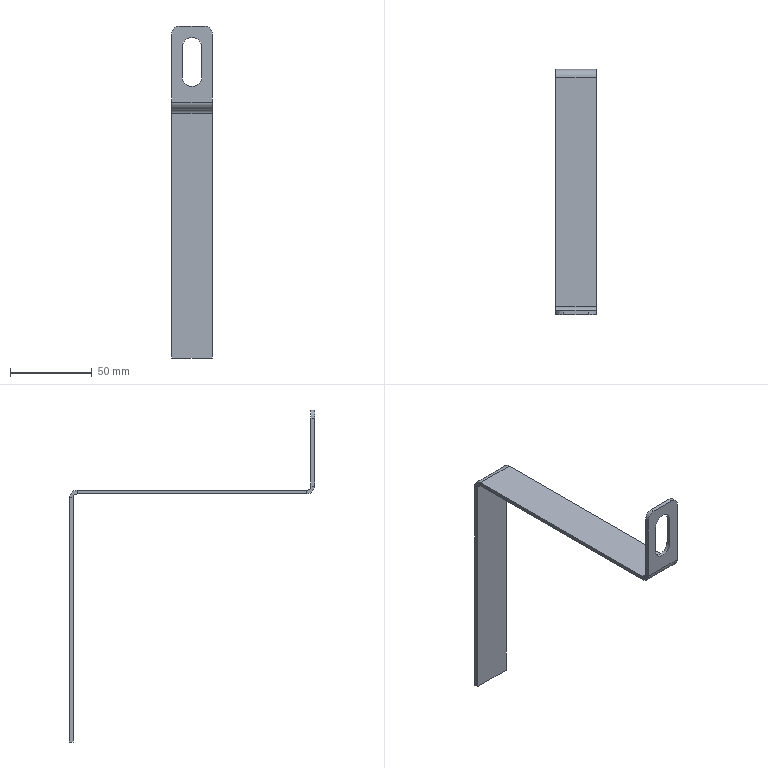Part | SolidWorks | features Fillet 1, FlatPattern 1, ICE 1, SMBaseFlange 1, SheetMetal 1 | 1 solid | 29 faces | box 25 x 150 x 203 mm | volume 19203 mm3 | plane 20 | cylinder 9 | commonest cylinder face diameters 12 x3 5 x2 9.6 x2 10 x2
STEP:
#1=CARTESIAN_POINT('',(6.,-2.3,-13.));
#2=VERTEX_POINT('',#1);
#3=CARTESIAN_POINT('',(0.,-2.3,-7.));
#4=VERTEX_POINT('',#3);
#5=CARTESIAN_POINT('',(0.,-2.3,-13.));
#6=DIRECTION('',(0.,-1.,0.));
#7=DIRECTION('',(0.,0.,1.));
#8=AXIS2_PLACEMENT_3D('',#5,#6,#7);
#9=CIRCLE('',#8,6.);
#10=EDGE_CURVE('',#2,#4,#9,.T.);
#11=ORIENTED_EDGE('',*,*,#10,.T.);
#12=CARTESIAN_POINT('',(0.,0.,-7.));
#13=VERTEX_POINT('',#12);
#14=CARTESIAN_POINT('',(0.,-2.301,-7.));
#15=DIRECTION('',(0.,1.,0.));
#16=VECTOR('',#15,1000.);
#17=LINE('',#14,#16);
#18=EDGE_CURVE('',#4,#13,#17,.T.);
#19=ORIENTED_EDGE('',*,*,#18,.T.);
#20=CARTESIAN_POINT('',(6.,0.,-13.));
#21=VERTEX_POINT('',#20);
#22=CARTESIAN_POINT('',(0.,0.,-13.));
#23=DIRECTION('',(0.,1.,0.));
#24=DIRECTION('',(0.,0.,1.));
#25=AXIS2_PLACEMENT_3D('',#22,#23,#24);
#26=CIRCLE('',#25,6.);
#27=EDGE_CURVE('',#13,#21,#26,.T.);
#28=ORIENTED_EDGE('',*,*,#27,.T.);
#29=CARTESIAN_POINT('',(6.,-2.301,-13.));
#30=DIRECTION('',(0.,1.,0.));
#31=VECTOR('',#30,1000.);
#32=LINE('',#29,#31);
#33=EDGE_CURVE('',#2,#21,#32,.T.);
#34=ORIENTED_EDGE('',*,*,#33,.F.);
#35=EDGE_LOOP('',(#11,#19,#28,#34));
#36=FACE_OUTER_BOUND('',#35,.T.);
#37=CARTESIAN_POINT('',(0.,-2.301,-13.));
#38=DIRECTION('',(0.,1.,0.));
#39=DIRECTION('',(0.,0.,1.));
#40=AXIS2_PLACEMENT_3D('',#37,#38,#39);
#41=CYLINDRICAL_SURFACE('',#40,6.);
#42=ADVANCED_FACE('',(#36),#41,.F.);
#43=CARTESIAN_POINT('',(12.5,2.5,-49.));
#44=VERTEX_POINT('',#43);
#45=CARTESIAN_POINT('',(12.5,2.5,-51.3));
#46=VERTEX_POINT('',#45);
#47=CARTESIAN_POINT('',(12.5,2.5,-49.));
#48=DIRECTION('',(0.,0.,-1.));
#49=VECTOR('',#48,1000.);
#50=LINE('',#47,#49);
#51=EDGE_CURVE('',#44,#46,#50,.T.);
#52=ORIENTED_EDGE('',*,*,#51,.F.);
#53=CARTESIAN_POINT('',(12.5,0.,-46.5));
#54=VERTEX_POINT('',#53);
#55=CARTESIAN_POINT('',(12.5,2.5,-46.5));
#56=DIRECTION('',(1.,0.,0.));
#57=DIRECTION('',(0.,0.,1.));
#58=AXIS2_PLACEMENT_3D('',#55,#56,#57);
#59=CIRCLE('',#58,2.5);
#60=EDGE_CURVE('',#54,#44,#59,.T.);
#61=ORIENTED_EDGE('',*,*,#60,.F.);
#62=CARTESIAN_POINT('',(12.5,-2.3,-46.5));
#63=VERTEX_POINT('',#62);
#64=CARTESIAN_POINT('',(12.5,-2.3,-46.5));
#65=DIRECTION('',(0.,1.,0.));
#66=VECTOR('',#65,1000.);
#67=LINE('',#64,#66);
#68=EDGE_CURVE('',#63,#54,#67,.T.);
#69=ORIENTED_EDGE('',*,*,#68,.F.);
#70=CARTESIAN_POINT('',(12.5,2.5,-46.5));
#71=DIRECTION('',(1.,0.,0.));
#72=DIRECTION('',(0.,0.,-1.));
#73=AXIS2_PLACEMENT_3D('',#70,#71,#72);
#74=CIRCLE('',#73,4.8);
#75=EDGE_CURVE('',#63,#46,#74,.T.);
#76=ORIENTED_EDGE('',*,*,#75,.T.);
#77=EDGE_LOOP('',(#52,#61,#69,#76));
#78=FACE_OUTER_BOUND('',#77,.T.);
#79=CARTESIAN_POINT('',(12.5,2.5,-49.));
#80=DIRECTION('',(1.,0.,0.));
#81=DIRECTION('',(0.,0.,-1.));
#82=AXIS2_PLACEMENT_3D('',#79,#80,#81);
#83=PLANE('',#82);
#84=ADVANCED_FACE('',(#78),#83,.T.);
#85=CARTESIAN_POINT('',(12.5,142.9,-49.));
#86=VERTEX_POINT('',#85);
#87=CARTESIAN_POINT('',(12.5,0.,-49.));
#88=DIRECTION('',(0.,1.,0.));
#89=VECTOR('',#88,1000.);
#90=LINE('',#87,#89);
#91=EDGE_CURVE('',#44,#86,#90,.T.);
#92=ORIENTED_EDGE('',*,*,#91,.F.);
#93=ORIENTED_EDGE('',*,*,#51,.T.);
#94=CARTESIAN_POINT('',(12.5,142.9,-51.3));
#95=VERTEX_POINT('',#94);
#96=CARTESIAN_POINT('',(12.5,0.,-51.3));
#97=DIRECTION('',(0.,1.,0.));
#98=VECTOR('',#97,1000.);
#99=LINE('',#96,#98);
#100=EDGE_CURVE('',#46,#95,#99,.T.);
#101=ORIENTED_EDGE('',*,*,#100,.T.);
#102=CARTESIAN_POINT('',(12.5,142.9,-51.3));
#103=DIRECTION('',(0.,0.,1.));
#104=VECTOR('',#103,1000.);
#105=LINE('',#102,#104);
#106=EDGE_CURVE('',#95,#86,#105,.T.);
#107=ORIENTED_EDGE('',*,*,#106,.T.);
#108=EDGE_LOOP('',(#92,#93,#101,#107));
#109=FACE_OUTER_BOUND('',#108,.T.);
#110=CARTESIAN_POINT('',(12.5,-2.3,-46.5));
#111=DIRECTION('',(1.,0.,0.));
#112=DIRECTION('',(0.,0.,-1.));
#113=AXIS2_PLACEMENT_3D('',#110,#111,#112);
#114=PLANE('',#113);
#115=ADVANCED_FACE('',(#109),#114,.T.);
#116=CARTESIAN_POINT('',(-12.5,0.,-46.5));
#117=VERTEX_POINT('',#116);
#118=CARTESIAN_POINT('',(-12.5,-2.3,-46.5));
#119=VERTEX_POINT('',#118);
#120=CARTESIAN_POINT('',(-12.5,0.,-46.5));
#121=DIRECTION('',(0.,-1.,0.));
#122=VECTOR('',#121,1000.);
#123=LINE('',#120,#122);
#124=EDGE_CURVE('',#117,#119,#123,.T.);
#125=ORIENTED_EDGE('',*,*,#124,.F.);
#126=CARTESIAN_POINT('',(-12.5,2.5,-49.));
#127=VERTEX_POINT('',#126);
#128=CARTESIAN_POINT('',(-12.5,2.5,-46.5));
#129=DIRECTION('',(1.,0.,0.));
#130=DIRECTION('',(0.,0.,1.));
#131=AXIS2_PLACEMENT_3D('',#128,#129,#130);
#132=CIRCLE('',#131,2.5);
#133=EDGE_CURVE('',#117,#127,#132,.T.);
#134=ORIENTED_EDGE('',*,*,#133,.T.);
#135=CARTESIAN_POINT('',(-12.5,2.5,-51.3));
#136=VERTEX_POINT('',#135);
#137=CARTESIAN_POINT('',(-12.5,2.5,-51.3));
#138=DIRECTION('',(0.,0.,1.));
#139=VECTOR('',#138,1000.);
#140=LINE('',#137,#139);
#141=EDGE_CURVE('',#136,#127,#140,.T.);
#142=ORIENTED_EDGE('',*,*,#141,.F.);
#143=CARTESIAN_POINT('',(-12.5,2.5,-46.5));
#144=DIRECTION('',(1.,0.,0.));
#145=DIRECTION('',(0.,0.,-1.));
#146=AXIS2_PLACEMENT_3D('',#143,#144,#145);
#147=CIRCLE('',#146,4.8);
#148=EDGE_CURVE('',#119,#136,#147,.T.);
#149=ORIENTED_EDGE('',*,*,#148,.F.);
#150=EDGE_LOOP('',(#125,#134,#142,#149));
#151=FACE_OUTER_BOUND('',#150,.T.);
#152=CARTESIAN_POINT('',(-12.5,0.,-46.5));
#153=DIRECTION('',(-1.,0.,0.));
#154=DIRECTION('',(0.,0.,1.));
#155=AXIS2_PLACEMENT_3D('',#152,#153,#154);
#156=PLANE('',#155);
#157=ADVANCED_FACE('',(#151),#156,.T.);
#158=CARTESIAN_POINT('',(-12.5,-2.3,-5.));
#159=VERTEX_POINT('',#158);
#160=CARTESIAN_POINT('',(-12.5,-2.3,0.));
#161=DIRECTION('',(0.,0.,-1.));
#162=VECTOR('',#161,1000.);
#163=LINE('',#160,#162);
#164=EDGE_CURVE('',#159,#119,#163,.T.);
#165=ORIENTED_EDGE('',*,*,#164,.F.);
#166=CARTESIAN_POINT('',(-12.5,0.,-5.));
#167=VERTEX_POINT('',#166);
#168=CARTESIAN_POINT('',(-12.5,2.5,-5.));
#169=DIRECTION('',(0.,1.,0.));
#170=VECTOR('',#169,1000.);
#171=LINE('',#168,#170);
#172=EDGE_CURVE('',#159,#167,#171,.T.);
#173=ORIENTED_EDGE('',*,*,#172,.T.);
#174=CARTESIAN_POINT('',(-12.5,0.,0.));
#175=DIRECTION('',(0.,0.,-1.));
#176=VECTOR('',#175,1000.);
#177=LINE('',#174,#176);
#178=EDGE_CURVE('',#167,#117,#177,.T.);
#179=ORIENTED_EDGE('',*,*,#178,.T.);
#180=ORIENTED_EDGE('',*,*,#124,.T.);
#181=EDGE_LOOP('',(#165,#173,#179,#180));
#182=FACE_OUTER_BOUND('',#181,.T.);
#183=CARTESIAN_POINT('',(-12.5,2.5,-51.3));
#184=DIRECTION('',(-1.,0.,0.));
#185=DIRECTION('',(0.,0.,1.));
#186=AXIS2_PLACEMENT_3D('',#183,#184,#185);
#187=PLANE('',#186);
#188=ADVANCED_FACE('',(#182),#187,.T.);
#189=CARTESIAN_POINT('',(12.5,147.7,-53.8));
#190=VERTEX_POINT('',#189);
#191=CARTESIAN_POINT('',(12.5,145.4,-53.8));
#192=VERTEX_POINT('',#191);
#193=CARTESIAN_POINT('',(12.5,147.7,-53.8));
#194=DIRECTION('',(0.,-1.,0.));
#195=VECTOR('',#194,1000.);
#196=LINE('',#193,#195);
#197=EDGE_CURVE('',#190,#192,#196,.T.);
#198=ORIENTED_EDGE('',*,*,#197,.F.);
#199=CARTESIAN_POINT('',(12.5,142.9,-53.8));
#200=DIRECTION('',(-1.,0.,0.));
#201=DIRECTION('',(0.,0.,-1.));
#202=AXIS2_PLACEMENT_3D('',#199,#200,#201);
#203=CIRCLE('',#202,4.8);
#204=EDGE_CURVE('',#86,#190,#203,.T.);
#205=ORIENTED_EDGE('',*,*,#204,.F.);
#206=ORIENTED_EDGE('',*,*,#106,.F.);
#207=CARTESIAN_POINT('',(12.5,142.9,-53.8));
#208=DIRECTION('',(-1.,0.,0.));
#209=DIRECTION('',(0.,0.,-1.));
#210=AXIS2_PLACEMENT_3D('',#207,#208,#209);
#211=CIRCLE('',#210,2.5);
#212=EDGE_CURVE('',#95,#192,#211,.T.);
#213=ORIENTED_EDGE('',*,*,#212,.T.);
#214=EDGE_LOOP('',(#198,#205,#206,#213));
#215=FACE_OUTER_BOUND('',#214,.T.);
#216=CARTESIAN_POINT('',(12.5,147.7,-53.8));
#217=DIRECTION('',(1.,0.,0.));
#218=DIRECTION('',(0.,0.,-1.));
#219=AXIS2_PLACEMENT_3D('',#216,#217,#218);
#220=PLANE('',#219);
#221=ADVANCED_FACE('',(#215),#220,.T.);
#222=CARTESIAN_POINT('',(12.5,147.7,-203.));
#223=VERTEX_POINT('',#222);
#224=CARTESIAN_POINT('',(12.5,147.7,-49.));
#225=DIRECTION('',(0.,0.,-1.));
#226=VECTOR('',#225,1000.);
#227=LINE('',#224,#226);
#228=EDGE_CURVE('',#190,#223,#227,.T.);
#229=ORIENTED_EDGE('',*,*,#228,.F.);
#230=ORIENTED_EDGE('',*,*,#197,.T.);
#231=CARTESIAN_POINT('',(12.5,145.4,-203.));
#232=VERTEX_POINT('',#231);
#233=CARTESIAN_POINT('',(12.5,145.4,-49.));
#234=DIRECTION('',(0.,0.,-1.));
#235=VECTOR('',#234,1000.);
#236=LINE('',#233,#235);
#237=EDGE_CURVE('',#192,#232,#236,.T.);
#238=ORIENTED_EDGE('',*,*,#237,.T.);
#239=CARTESIAN_POINT('',(12.5,147.7,-203.));
#240=DIRECTION('',(0.,-1.,0.));
#241=VECTOR('',#240,1000.);
#242=LINE('',#239,#241);
#243=EDGE_CURVE('',#223,#232,#242,.T.);
#244=ORIENTED_EDGE('',*,*,#243,.F.);
#245=EDGE_LOOP('',(#229,#230,#238,#244));
#246=FACE_OUTER_BOUND('',#245,.T.);
#247=CARTESIAN_POINT('',(12.5,142.9,-51.3));
#248=DIRECTION('',(1.,0.,0.));
#249=DIRECTION('',(0.,0.,-1.));
#250=AXIS2_PLACEMENT_3D('',#247,#248,#249);
#251=PLANE('',#250);
#252=ADVANCED_FACE('',(#246),#251,.T.);
#253=CARTESIAN_POINT('',(-12.5,142.9,-49.));
#254=VERTEX_POINT('',#253);
#255=CARTESIAN_POINT('',(-12.5,142.9,-51.3));
#256=VERTEX_POINT('',#255);
#257=CARTESIAN_POINT('',(-12.5,142.9,-49.));
#258=DIRECTION('',(0.,0.,-1.));
#259=VECTOR('',#258,1000.);
#260=LINE('',#257,#259);
#261=EDGE_CURVE('',#254,#256,#260,.T.);
#262=ORIENTED_EDGE('',*,*,#261,.F.);
#263=CARTESIAN_POINT('',(-12.5,147.7,-53.8));
#264=VERTEX_POINT('',#263);
#265=CARTESIAN_POINT('',(-12.5,142.9,-53.8));
#266=DIRECTION('',(-1.,0.,0.));
#267=DIRECTION('',(0.,0.,-1.));
#268=AXIS2_PLACEMENT_3D('',#265,#266,#267);
#269=CIRCLE('',#268,4.8);
#270=EDGE_CURVE('',#254,#264,#269,.T.);
#271=ORIENTED_EDGE('',*,*,#270,.T.);
#272=CARTESIAN_POINT('',(-12.5,145.4,-53.8));
#273=VERTEX_POINT('',#272);
#274=CARTESIAN_POINT('',(-12.5,145.4,-53.8));
#275=DIRECTION('',(0.,1.,0.));
#276=VECTOR('',#275,1000.);
#277=LINE('',#274,#276);
#278=EDGE_CURVE('',#273,#264,#277,.T.);
#279=ORIENTED_EDGE('',*,*,#278,.F.);
#280=CARTESIAN_POINT('',(-12.5,142.9,-53.8));
#281=DIRECTION('',(-1.,0.,0.));
#282=DIRECTION('',(0.,0.,-1.));
#283=AXIS2_PLACEMENT_3D('',#280,#281,#282);
#284=CIRCLE('',#283,2.5);
#285=EDGE_CURVE('',#256,#273,#284,.T.);
#286=ORIENTED_EDGE('',*,*,#285,.F.);
#287=EDGE_LOOP('',(#262,#271,#279,#286));
#288=FACE_OUTER_BOUND('',#287,.T.);
#289=CARTESIAN_POINT('',(-12.5,142.9,-49.));
#290=DIRECTION('',(-1.,0.,0.));
#291=DIRECTION('',(0.,0.,1.));
#292=AXIS2_PLACEMENT_3D('',#289,#290,#291);
#293=PLANE('',#292);
#294=ADVANCED_FACE('',(#288),#293,.T.);
#295=CARTESIAN_POINT('',(-12.5,0.,-49.));
#296=DIRECTION('',(0.,1.,0.));
#297=VECTOR('',#296,1000.);
#298=LINE('',#295,#297);
#299=EDGE_CURVE('',#127,#254,#298,.T.);
#300=ORIENTED_EDGE('',*,*,#299,.T.);
#301=ORIENTED_EDGE('',*,*,#261,.T.);
#302=CARTESIAN_POINT('',(-12.5,0.,-51.3));
#303=DIRECTION('',(0.,1.,0.));
#304=VECTOR('',#303,1000.);
#305=LINE('',#302,#304);
#306=EDGE_CURVE('',#136,#256,#305,.T.);
#307=ORIENTED_EDGE('',*,*,#306,.F.);
#308=ORIENTED_EDGE('',*,*,#141,.T.);
#309=EDGE_LOOP('',(#300,#301,#307,#308));
#310=FACE_OUTER_BOUND('',#309,.T.);
#311=CARTESIAN_POINT('',(-12.5,145.4,-53.8));
#312=DIRECTION('',(-1.,0.,0.));
#313=DIRECTION('',(0.,0.,1.));
#314=AXIS2_PLACEMENT_3D('',#311,#312,#313);
#315=PLANE('',#314);
#316=ADVANCED_FACE('',(#310),#315,.T.);
#317=CARTESIAN_POINT('',(-12.5,145.4,-203.));
#318=VERTEX_POINT('',#317);
#319=CARTESIAN_POINT('',(-12.5,145.4,-49.));
#320=DIRECTION('',(0.,0.,-1.));
#321=VECTOR('',#320,1000.);
#322=LINE('',#319,#321);
#323=EDGE_CURVE('',#273,#318,#322,.T.);
#324=ORIENTED_EDGE('',*,*,#323,.T.);
#325=CARTESIAN_POINT('',(12.5,145.4,-203.));
#326=DIRECTION('',(-1.,0.,0.));
#327=VECTOR('',#326,1000.);
#328=LINE('',#325,#327);
#329=EDGE_CURVE('',#232,#318,#328,.T.);
#330=ORIENTED_EDGE('',*,*,#329,.F.);
#331=ORIENTED_EDGE('',*,*,#237,.F.);
#332=CARTESIAN_POINT('',(12.5,145.4,-53.8));
#333=DIRECTION('',(-1.,0.,0.));
#334=VECTOR('',#333,1000.);
#335=LINE('',#332,#334);
#336=EDGE_CURVE('',#192,#273,#335,.T.);
#337=ORIENTED_EDGE('',*,*,#336,.T.);
#338=EDGE_LOOP('',(#324,#330,#331,#337));
#339=FACE_OUTER_BOUND('',#338,.T.);
#340=CARTESIAN_POINT('',(12.5,145.4,-49.));
#341=DIRECTION('',(0.,1.,0.));
#342=DIRECTION('',(0.,0.,1.));
#343=AXIS2_PLACEMENT_3D('',#340,#341,#342);
#344=PLANE('',#343);
#345=ADVANCED_FACE('',(#339),#344,.F.);
#346=CARTESIAN_POINT('',(-12.5,147.7,-203.));
#347=VERTEX_POINT('',#346);
#348=CARTESIAN_POINT('',(-12.5,147.7,-203.));
#349=DIRECTION('',(0.,-1.,0.));
#350=VECTOR('',#349,1000.);
#351=LINE('',#348,#350);
#352=EDGE_CURVE('',#347,#318,#351,.T.);
#353=ORIENTED_EDGE('',*,*,#352,.F.);
#354=CARTESIAN_POINT('',(12.5,147.7,-203.));
#355=DIRECTION('',(-1.,0.,0.));
#356=VECTOR('',#355,1000.);
#357=LINE('',#354,#356);
#358=EDGE_CURVE('',#223,#347,#357,.T.);
#359=ORIENTED_EDGE('',*,*,#358,.F.);
#360=ORIENTED_EDGE('',*,*,#243,.T.);
#361=ORIENTED_EDGE('',*,*,#329,.T.);
#362=EDGE_LOOP('',(#353,#359,#360,#361));
#363=FACE_OUTER_BOUND('',#362,.T.);
#364=CARTESIAN_POINT('',(12.5,147.7,-203.));
#365=DIRECTION('',(0.,0.,-1.));
#366=DIRECTION('',(-1.,0.,0.));
#367=AXIS2_PLACEMENT_3D('',#364,#365,#366);
#368=PLANE('',#367);
#369=ADVANCED_FACE('',(#363),#368,.T.);
#370=CARTESIAN_POINT('',(-12.5,147.7,-49.));
#371=DIRECTION('',(0.,0.,-1.));
#372=VECTOR('',#371,1000.);
#373=LINE('',#370,#372);
#374=EDGE_CURVE('',#264,#347,#373,.T.);
#375=ORIENTED_EDGE('',*,*,#374,.F.);
#376=CARTESIAN_POINT('',(12.5,147.7,-53.8));
#377=DIRECTION('',(-1.,0.,0.));
#378=VECTOR('',#377,1000.);
#379=LINE('',#376,#378);
#380=EDGE_CURVE('',#190,#264,#379,.T.);
#381=ORIENTED_EDGE('',*,*,#380,.F.);
#382=ORIENTED_EDGE('',*,*,#228,.T.);
#383=ORIENTED_EDGE('',*,*,#358,.T.);
#384=EDGE_LOOP('',(#375,#381,#382,#383));
#385=FACE_OUTER_BOUND('',#384,.T.);
#386=CARTESIAN_POINT('',(12.5,147.7,-49.));
#387=DIRECTION('',(0.,1.,0.));
#388=DIRECTION('',(0.,0.,1.));
#389=AXIS2_PLACEMENT_3D('',#386,#387,#388);
#390=PLANE('',#389);
#391=ADVANCED_FACE('',(#385),#390,.T.);
#392=ORIENTED_EDGE('',*,*,#270,.F.);
#393=CARTESIAN_POINT('',(12.5,142.9,-49.));
#394=DIRECTION('',(-1.,0.,0.));
#395=VECTOR('',#394,1000.);
#396=LINE('',#393,#395);
#397=EDGE_CURVE('',#86,#254,#396,.T.);
#398=ORIENTED_EDGE('',*,*,#397,.F.);
#399=ORIENTED_EDGE('',*,*,#204,.T.);
#400=ORIENTED_EDGE('',*,*,#380,.T.);
#401=EDGE_LOOP('',(#392,#398,#399,#400));
#402=FACE_OUTER_BOUND('',#401,.T.);
#403=CARTESIAN_POINT('',(12.5,142.9,-53.8));
#404=DIRECTION('',(-1.,0.,0.));
#405=DIRECTION('',(0.,0.,1.));
#406=AXIS2_PLACEMENT_3D('',#403,#404,#405);
#407=CYLINDRICAL_SURFACE('',#406,4.8);
#408=ADVANCED_FACE('',(#402),#407,.T.);
#409=ORIENTED_EDGE('',*,*,#299,.F.);
#410=CARTESIAN_POINT('',(12.5,2.5,-49.));
#411=DIRECTION('',(-1.,0.,0.));
#412=VECTOR('',#411,1000.);
#413=LINE('',#410,#412);
#414=EDGE_CURVE('',#44,#127,#413,.T.);
#415=ORIENTED_EDGE('',*,*,#414,.F.);
#416=ORIENTED_EDGE('',*,*,#91,.T.);
#417=ORIENTED_EDGE('',*,*,#397,.T.);
#418=EDGE_LOOP('',(#409,#415,#416,#417));
#419=FACE_OUTER_BOUND('',#418,.T.);
#420=CARTESIAN_POINT('',(12.5,0.,-49.));
#421=DIRECTION('',(0.,0.,1.));
#422=DIRECTION('',(1.,0.,0.));
#423=AXIS2_PLACEMENT_3D('',#420,#421,#422);
#424=PLANE('',#423);
#425=ADVANCED_FACE('',(#419),#424,.T.);
#426=ORIENTED_EDGE('',*,*,#133,.F.);
#427=CARTESIAN_POINT('',(12.5,0.,-46.5));
#428=DIRECTION('',(-1.,0.,0.));
#429=VECTOR('',#428,1000.);
#430=LINE('',#427,#429);
#431=EDGE_CURVE('',#54,#117,#430,.T.);
#432=ORIENTED_EDGE('',*,*,#431,.F.);
#433=ORIENTED_EDGE('',*,*,#60,.T.);
#434=ORIENTED_EDGE('',*,*,#414,.T.);
#435=EDGE_LOOP('',(#426,#432,#433,#434));
#436=FACE_OUTER_BOUND('',#435,.T.);
#437=CARTESIAN_POINT('',(12.5,2.5,-46.5));
#438=DIRECTION('',(-1.,0.,0.));
#439=DIRECTION('',(0.,0.,1.));
#440=AXIS2_PLACEMENT_3D('',#437,#438,#439);
#441=CYLINDRICAL_SURFACE('',#440,2.5);
#442=ADVANCED_FACE('',(#436),#441,.F.);
#443=CARTESIAN_POINT('',(6.,0.,-31.));
#444=VERTEX_POINT('',#443);
#445=CARTESIAN_POINT('',(-6.,0.,-31.));
#446=VERTEX_POINT('',#445);
#447=CARTESIAN_POINT('',(0.,0.,-31.));
#448=DIRECTION('',(0.,1.,0.));
#449=DIRECTION('',(0.,0.,1.));
#450=AXIS2_PLACEMENT_3D('',#447,#448,#449);
#451=CIRCLE('',#450,6.);
#452=EDGE_CURVE('',#444,#446,#451,.T.);
#453=ORIENTED_EDGE('',*,*,#452,.F.);
#454=CARTESIAN_POINT('',(6.,0.,-31.));
#455=DIRECTION('',(0.,0.,-1.));
#456=VECTOR('',#455,1000.);
#457=LINE('',#454,#456);
#458=EDGE_CURVE('',#21,#444,#457,.T.);
#459=ORIENTED_EDGE('',*,*,#458,.F.);
#460=ORIENTED_EDGE('',*,*,#27,.F.);
#461=CARTESIAN_POINT('',(-6.,0.,-13.));
#462=VERTEX_POINT('',#461);
#463=CARTESIAN_POINT('',(0.,0.,-13.));
#464=DIRECTION('',(0.,1.,0.));
#465=DIRECTION('',(0.,0.,1.));
#466=AXIS2_PLACEMENT_3D('',#463,#464,#465);
#467=CIRCLE('',#466,6.);
#468=EDGE_CURVE('',#462,#13,#467,.T.);
#469=ORIENTED_EDGE('',*,*,#468,.F.);
#470=CARTESIAN_POINT('',(-6.,0.,-31.));
#471=DIRECTION('',(0.,0.,1.));
#472=VECTOR('',#471,1000.);
#473=LINE('',#470,#472);
#474=EDGE_CURVE('',#446,#462,#473,.T.);
#475=ORIENTED_EDGE('',*,*,#474,.F.);
#476=EDGE_LOOP('',(#453,#459,#460,#469,#475));
#477=FACE_BOUND('',#476,.T.);
#478=CARTESIAN_POINT('',(7.5,0.,0.));
#479=VERTEX_POINT('',#478);
#480=CARTESIAN_POINT('',(-7.5,0.,0.));
#481=VERTEX_POINT('',#480);
#482=CARTESIAN_POINT('',(12.5,0.,0.));
#483=DIRECTION('',(-1.,0.,0.));
#484=VECTOR('',#483,1000.);
#485=LINE('',#482,#484);
#486=EDGE_CURVE('',#479,#481,#485,.T.);
#487=ORIENTED_EDGE('',*,*,#486,.F.);
#488=CARTESIAN_POINT('',(12.5,0.,-5.));
#489=VERTEX_POINT('',#488);
#490=CARTESIAN_POINT('',(7.5,0.,-5.));
#491=DIRECTION('',(0.,1.,0.));
#492=DIRECTION('',(0.,0.,1.));
#493=AXIS2_PLACEMENT_3D('',#490,#491,#492);
#494=CIRCLE('',#493,5.);
#495=EDGE_CURVE('',#479,#489,#494,.T.);
#496=ORIENTED_EDGE('',*,*,#495,.T.);
#497=CARTESIAN_POINT('',(12.5,0.,0.));
#498=DIRECTION('',(0.,0.,-1.));
#499=VECTOR('',#498,1000.);
#500=LINE('',#497,#499);
#501=EDGE_CURVE('',#489,#54,#500,.T.);
#502=ORIENTED_EDGE('',*,*,#501,.T.);
#503=ORIENTED_EDGE('',*,*,#431,.T.);
#504=ORIENTED_EDGE('',*,*,#178,.F.);
#505=CARTESIAN_POINT('',(-7.5,0.,-5.));
#506=DIRECTION('',(0.,1.,0.));
#507=DIRECTION('',(0.,0.,1.));
#508=AXIS2_PLACEMENT_3D('',#505,#506,#507);
#509=CIRCLE('',#508,5.);
#510=EDGE_CURVE('',#167,#481,#509,.T.);
#511=ORIENTED_EDGE('',*,*,#510,.T.);
#512=EDGE_LOOP('',(#487,#496,#502,#503,#504,#511));
#513=FACE_OUTER_BOUND('',#512,.T.);
#514=CARTESIAN_POINT('',(12.5,0.,0.));
#515=DIRECTION('',(0.,1.,0.));
#516=DIRECTION('',(0.,0.,1.));
#517=AXIS2_PLACEMENT_3D('',#514,#515,#516);
#518=PLANE('',#517);
#519=ADVANCED_FACE('',(#477,#513),#518,.T.);
#520=CARTESIAN_POINT('',(7.5,-2.3,0.));
#521=VERTEX_POINT('',#520);
#522=CARTESIAN_POINT('',(-7.5,-2.3,0.));
#523=VERTEX_POINT('',#522);
#524=CARTESIAN_POINT('',(12.5,-2.3,0.));
#525=DIRECTION('',(-1.,0.,0.));
#526=VECTOR('',#525,1000.);
#527=LINE('',#524,#526);
#528=EDGE_CURVE('',#521,#523,#527,.T.);
#529=ORIENTED_EDGE('',*,*,#528,.F.);
#530=CARTESIAN_POINT('',(7.5,-2.3,0.));
#531=DIRECTION('',(0.,1.,0.));
#532=VECTOR('',#531,1000.);
#533=LINE('',#530,#532);
#534=EDGE_CURVE('',#521,#479,#533,.T.);
#535=ORIENTED_EDGE('',*,*,#534,.T.);
#536=ORIENTED_EDGE('',*,*,#486,.T.);
#537=CARTESIAN_POINT('',(-7.5,-2.3,0.));
#538=DIRECTION('',(0.,-1.,0.));
#539=VECTOR('',#538,1000.);
#540=LINE('',#537,#539);
#541=EDGE_CURVE('',#481,#523,#540,.T.);
#542=ORIENTED_EDGE('',*,*,#541,.T.);
#543=EDGE_LOOP('',(#529,#535,#536,#542));
#544=FACE_OUTER_BOUND('',#543,.T.);
#545=CARTESIAN_POINT('',(12.5,-2.3,0.));
#546=DIRECTION('',(0.,0.,1.));
#547=DIRECTION('',(1.,0.,0.));
#548=AXIS2_PLACEMENT_3D('',#545,#546,#547);
#549=PLANE('',#548);
#550=ADVANCED_FACE('',(#544),#549,.T.);
#551=CARTESIAN_POINT('',(6.,-2.3,-31.));
#552=VERTEX_POINT('',#551);
#553=CARTESIAN_POINT('',(6.,-2.3,-31.));
#554=DIRECTION('',(0.,0.,1.));
#555=VECTOR('',#554,1000.);
#556=LINE('',#553,#555);
#557=EDGE_CURVE('',#552,#2,#556,.T.);
#558=ORIENTED_EDGE('',*,*,#557,.F.);
#559=CARTESIAN_POINT('',(-6.,-2.3,-31.));
#560=VERTEX_POINT('',#559);
#561=CARTESIAN_POINT('',(0.,-2.3,-31.));
#562=DIRECTION('',(0.,-1.,0.));
#563=DIRECTION('',(0.,0.,1.));
#564=AXIS2_PLACEMENT_3D('',#561,#562,#563);
#565=CIRCLE('',#564,6.);
#566=EDGE_CURVE('',#560,#552,#565,.T.);
#567=ORIENTED_EDGE('',*,*,#566,.F.);
#568=CARTESIAN_POINT('',(-6.,-2.3,-13.));
#569=VERTEX_POINT('',#568);
#570=CARTESIAN_POINT('',(-6.,-2.3,-31.));
#571=DIRECTION('',(0.,0.,-1.));
#572=VECTOR('',#571,1000.);
#573=LINE('',#570,#572);
#574=EDGE_CURVE('',#569,#560,#573,.T.);
#575=ORIENTED_EDGE('',*,*,#574,.F.);
#576=CARTESIAN_POINT('',(0.,-2.3,-13.));
#577=DIRECTION('',(0.,-1.,0.));
#578=DIRECTION('',(0.,0.,1.));
#579=AXIS2_PLACEMENT_3D('',#576,#577,#578);
#580=CIRCLE('',#579,6.);
#581=EDGE_CURVE('',#4,#569,#580,.T.);
#582=ORIENTED_EDGE('',*,*,#581,.F.);
#583=ORIENTED_EDGE('',*,*,#10,.F.);
#584=EDGE_LOOP('',(#558,#567,#575,#582,#583));
#585=FACE_BOUND('',#584,.T.);
#586=CARTESIAN_POINT('',(12.5,-2.3,-5.));
#587=VERTEX_POINT('',#586);
#588=CARTESIAN_POINT('',(12.5,-2.3,0.));
#589=DIRECTION('',(0.,0.,-1.));
#590=VECTOR('',#589,1000.);
#591=LINE('',#588,#590);
#592=EDGE_CURVE('',#587,#63,#591,.T.);
#593=ORIENTED_EDGE('',*,*,#592,.F.);
#594=CARTESIAN_POINT('',(7.5,-2.3,-5.));
#595=DIRECTION('',(0.,-1.,0.));
#596=DIRECTION('',(0.,0.,1.));
#597=AXIS2_PLACEMENT_3D('',#594,#595,#596);
#598=CIRCLE('',#597,5.);
#599=EDGE_CURVE('',#587,#521,#598,.T.);
#600=ORIENTED_EDGE('',*,*,#599,.T.);
#601=ORIENTED_EDGE('',*,*,#528,.T.);
#602=CARTESIAN_POINT('',(-7.5,-2.3,-5.));
#603=DIRECTION('',(0.,-1.,0.));
#604=DIRECTION('',(0.,0.,1.));
#605=AXIS2_PLACEMENT_3D('',#602,#603,#604);
#606=CIRCLE('',#605,5.);
#607=EDGE_CURVE('',#523,#159,#606,.T.);
#608=ORIENTED_EDGE('',*,*,#607,.T.);
#609=ORIENTED_EDGE('',*,*,#164,.T.);
#610=CARTESIAN_POINT('',(12.5,-2.3,-46.5));
#611=DIRECTION('',(-1.,0.,0.));
#612=VECTOR('',#611,1000.);
#613=LINE('',#610,#612);
#614=EDGE_CURVE('',#63,#119,#613,.T.);
#615=ORIENTED_EDGE('',*,*,#614,.F.);
#616=EDGE_LOOP('',(#593,#600,#601,#608,#609,#615));
#617=FACE_OUTER_BOUND('',#616,.T.);
#618=CARTESIAN_POINT('',(12.5,-2.3,0.));
#619=DIRECTION('',(0.,1.,0.));
#620=DIRECTION('',(0.,0.,1.));
#621=AXIS2_PLACEMENT_3D('',#618,#619,#620);
#622=PLANE('',#621);
#623=ADVANCED_FACE('',(#585,#617),#622,.F.);
#624=ORIENTED_EDGE('',*,*,#148,.T.);
#625=CARTESIAN_POINT('',(12.5,2.5,-51.3));
#626=DIRECTION('',(-1.,0.,0.));
#627=VECTOR('',#626,1000.);
#628=LINE('',#625,#627);
#629=EDGE_CURVE('',#46,#136,#628,.T.);
#630=ORIENTED_EDGE('',*,*,#629,.F.);
#631=ORIENTED_EDGE('',*,*,#75,.F.);
#632=ORIENTED_EDGE('',*,*,#614,.T.);
#633=EDGE_LOOP('',(#624,#630,#631,#632));
#634=FACE_OUTER_BOUND('',#633,.T.);
#635=CARTESIAN_POINT('',(12.5,2.5,-46.5));
#636=DIRECTION('',(-1.,0.,0.));
#637=DIRECTION('',(0.,0.,1.));
#638=AXIS2_PLACEMENT_3D('',#635,#636,#637);
#639=CYLINDRICAL_SURFACE('',#638,4.8);
#640=ADVANCED_FACE('',(#634),#639,.T.);
#641=ORIENTED_EDGE('',*,*,#306,.T.);
#642=CARTESIAN_POINT('',(12.5,142.9,-51.3));
#643=DIRECTION('',(-1.,0.,0.));
#644=VECTOR('',#643,1000.);
#645=LINE('',#642,#644);
#646=EDGE_CURVE('',#95,#256,#645,.T.);
#647=ORIENTED_EDGE('',*,*,#646,.F.);
#648=ORIENTED_EDGE('',*,*,#100,.F.);
#649=ORIENTED_EDGE('',*,*,#629,.T.);
#650=EDGE_LOOP('',(#641,#647,#648,#649));
#651=FACE_OUTER_BOUND('',#650,.T.);
#652=CARTESIAN_POINT('',(12.5,0.,-51.3));
#653=DIRECTION('',(0.,0.,1.));
#654=DIRECTION('',(1.,0.,0.));
#655=AXIS2_PLACEMENT_3D('',#652,#653,#654);
#656=PLANE('',#655);
#657=ADVANCED_FACE('',(#651),#656,.F.);
#658=ORIENTED_EDGE('',*,*,#285,.T.);
#659=ORIENTED_EDGE('',*,*,#336,.F.);
#660=ORIENTED_EDGE('',*,*,#212,.F.);
#661=ORIENTED_EDGE('',*,*,#646,.T.);
#662=EDGE_LOOP('',(#658,#659,#660,#661));
#663=FACE_OUTER_BOUND('',#662,.T.);
#664=CARTESIAN_POINT('',(12.5,142.9,-53.8));
#665=DIRECTION('',(-1.,0.,0.));
#666=DIRECTION('',(0.,0.,1.));
#667=AXIS2_PLACEMENT_3D('',#664,#665,#666);
#668=CYLINDRICAL_SURFACE('',#667,2.5);
#669=ADVANCED_FACE('',(#663),#668,.F.);
#670=ORIENTED_EDGE('',*,*,#501,.F.);
#671=CARTESIAN_POINT('',(12.5,142.9,-5.));
#672=DIRECTION('',(0.,-1.,0.));
#673=VECTOR('',#672,1000.);
#674=LINE('',#671,#673);
#675=EDGE_CURVE('',#489,#587,#674,.T.);
#676=ORIENTED_EDGE('',*,*,#675,.T.);
#677=ORIENTED_EDGE('',*,*,#592,.T.);
#678=ORIENTED_EDGE('',*,*,#68,.T.);
#679=EDGE_LOOP('',(#670,#676,#677,#678));
#680=FACE_OUTER_BOUND('',#679,.T.);
#681=CARTESIAN_POINT('',(12.5,142.9,-53.8));
#682=DIRECTION('',(1.,0.,0.));
#683=DIRECTION('',(0.,0.,-1.));
#684=AXIS2_PLACEMENT_3D('',#681,#682,#683);
#685=PLANE('',#684);
#686=ADVANCED_FACE('',(#680),#685,.T.);
#687=ORIENTED_EDGE('',*,*,#323,.F.);
#688=ORIENTED_EDGE('',*,*,#278,.T.);
#689=ORIENTED_EDGE('',*,*,#374,.T.);
#690=ORIENTED_EDGE('',*,*,#352,.T.);
#691=EDGE_LOOP('',(#687,#688,#689,#690));
#692=FACE_OUTER_BOUND('',#691,.T.);
#693=CARTESIAN_POINT('',(-12.5,142.9,-53.8));
#694=DIRECTION('',(1.,0.,0.));
#695=DIRECTION('',(0.,0.,-1.));
#696=AXIS2_PLACEMENT_3D('',#693,#694,#695);
#697=PLANE('',#696);
#698=ADVANCED_FACE('',(#692),#697,.F.);
#699=ORIENTED_EDGE('',*,*,#566,.T.);
#700=CARTESIAN_POINT('',(6.,-2.301,-31.));
#701=DIRECTION('',(0.,1.,0.));
#702=VECTOR('',#701,1000.);
#703=LINE('',#700,#702);
#704=EDGE_CURVE('',#552,#444,#703,.T.);
#705=ORIENTED_EDGE('',*,*,#704,.T.);
#706=ORIENTED_EDGE('',*,*,#452,.T.);
#707=CARTESIAN_POINT('',(-6.,-2.301,-31.));
#708=DIRECTION('',(0.,1.,0.));
#709=VECTOR('',#708,1000.);
#710=LINE('',#707,#709);
#711=EDGE_CURVE('',#560,#446,#710,.T.);
#712=ORIENTED_EDGE('',*,*,#711,.F.);
#713=EDGE_LOOP('',(#699,#705,#706,#712));
#714=FACE_OUTER_BOUND('',#713,.T.);
#715=CARTESIAN_POINT('',(0.,-2.301,-31.));
#716=DIRECTION('',(0.,1.,0.));
#717=DIRECTION('',(0.,0.,1.));
#718=AXIS2_PLACEMENT_3D('',#715,#716,#717);
#719=CYLINDRICAL_SURFACE('',#718,6.);
#720=ADVANCED_FACE('',(#714),#719,.F.);
#721=ORIENTED_EDGE('',*,*,#557,.T.);
#722=ORIENTED_EDGE('',*,*,#33,.T.);
#723=ORIENTED_EDGE('',*,*,#458,.T.);
#724=ORIENTED_EDGE('',*,*,#704,.F.);
#725=EDGE_LOOP('',(#721,#722,#723,#724));
#726=FACE_OUTER_BOUND('',#725,.T.);
#727=CARTESIAN_POINT('',(6.,-2.301,-31.));
#728=DIRECTION('',(1.,0.,0.));
#729=DIRECTION('',(0.,0.,-1.));
#730=AXIS2_PLACEMENT_3D('',#727,#728,#729);
#731=PLANE('',#730);
#732=ADVANCED_FACE('',(#726),#731,.F.);
#733=ORIENTED_EDGE('',*,*,#18,.F.);
#734=ORIENTED_EDGE('',*,*,#581,.T.);
#735=CARTESIAN_POINT('',(-6.,-2.301,-13.));
#736=DIRECTION('',(0.,1.,0.));
#737=VECTOR('',#736,1000.);
#738=LINE('',#735,#737);
#739=EDGE_CURVE('',#569,#462,#738,.T.);
#740=ORIENTED_EDGE('',*,*,#739,.T.);
#741=ORIENTED_EDGE('',*,*,#468,.T.);
#742=EDGE_LOOP('',(#733,#734,#740,#741));
#743=FACE_OUTER_BOUND('',#742,.T.);
#744=CARTESIAN_POINT('',(0.,-2.301,-13.));
#745=DIRECTION('',(0.,1.,0.));
#746=DIRECTION('',(0.,0.,1.));
#747=AXIS2_PLACEMENT_3D('',#744,#745,#746);
#748=CYLINDRICAL_SURFACE('',#747,6.);
#749=ADVANCED_FACE('',(#743),#748,.F.);
#750=ORIENTED_EDGE('',*,*,#574,.T.);
#751=ORIENTED_EDGE('',*,*,#711,.T.);
#752=ORIENTED_EDGE('',*,*,#474,.T.);
#753=ORIENTED_EDGE('',*,*,#739,.F.);
#754=EDGE_LOOP('',(#750,#751,#752,#753));
#755=FACE_OUTER_BOUND('',#754,.T.);
#756=CARTESIAN_POINT('',(-6.,-2.301,-31.));
#757=DIRECTION('',(-1.,0.,0.));
#758=DIRECTION('',(0.,0.,1.));
#759=AXIS2_PLACEMENT_3D('',#756,#757,#758);
#760=PLANE('',#759);
#761=ADVANCED_FACE('',(#755),#760,.F.);
#762=ORIENTED_EDGE('',*,*,#599,.F.);
#763=ORIENTED_EDGE('',*,*,#675,.F.);
#764=ORIENTED_EDGE('',*,*,#495,.F.);
#765=ORIENTED_EDGE('',*,*,#534,.F.);
#766=EDGE_LOOP('',(#762,#763,#764,#765));
#767=FACE_OUTER_BOUND('',#766,.T.);
#768=CARTESIAN_POINT('',(7.5,-2.3,-5.));
#769=DIRECTION('',(0.,1.,0.));
#770=DIRECTION('',(0.,0.,1.));
#771=AXIS2_PLACEMENT_3D('',#768,#769,#770);
#772=CYLINDRICAL_SURFACE('',#771,5.);
#773=ADVANCED_FACE('',(#767),#772,.T.);
#774=ORIENTED_EDGE('',*,*,#607,.F.);
#775=ORIENTED_EDGE('',*,*,#541,.F.);
#776=ORIENTED_EDGE('',*,*,#510,.F.);
#777=ORIENTED_EDGE('',*,*,#172,.F.);
#778=EDGE_LOOP('',(#774,#775,#776,#777));
#779=FACE_OUTER_BOUND('',#778,.T.);
#780=CARTESIAN_POINT('',(-7.5,2.5,-5.));
#781=DIRECTION('',(0.,1.,0.));
#782=DIRECTION('',(0.,0.,1.));
#783=AXIS2_PLACEMENT_3D('',#780,#781,#782);
#784=CYLINDRICAL_SURFACE('',#783,5.);
#785=ADVANCED_FACE('',(#779),#784,.T.);
#786=CLOSED_SHELL('',(#42,#84,#115,#157,#188,#221,#252,#294,#316,#345,#369,#391,#408,#425,#442,#519,#550,#623,#640,#657,#669,#686,#698,#720,#732,#749,#761,#773,#785));
#787=MANIFOLD_SOLID_BREP('',#786);
#788=CARTESIAN_POINT('',(0.,0.,0.));
#789=DIRECTION('',(0.,0.,1.));
#790=DIRECTION('',(1.,0.,0.));
#791=AXIS2_PLACEMENT_3D('',#788,#789,#790);
#792=(LENGTH_UNIT()NAMED_UNIT(*)SI_UNIT(.MILLI.,.METRE.));
#793=UNCERTAINTY_MEASURE_WITH_UNIT(LENGTH_MEASURE(0.00001),#792,'','');
#794=(NAMED_UNIT(*)PLANE_ANGLE_UNIT()SI_UNIT($,.RADIAN.));
#795=(NAMED_UNIT(*)SI_UNIT($,.STERADIAN.)SOLID_ANGLE_UNIT());
#796=(GEOMETRIC_REPRESENTATION_CONTEXT(3)GLOBAL_UNCERTAINTY_ASSIGNED_CONTEXT((#793))GLOBAL_UNIT_ASSIGNED_CONTEXT((#792,#794,#795))REPRESENTATION_CONTEXT('',''));
#797=ADVANCED_BREP_SHAPE_REPRESENTATION('',(#787,#791),#796);